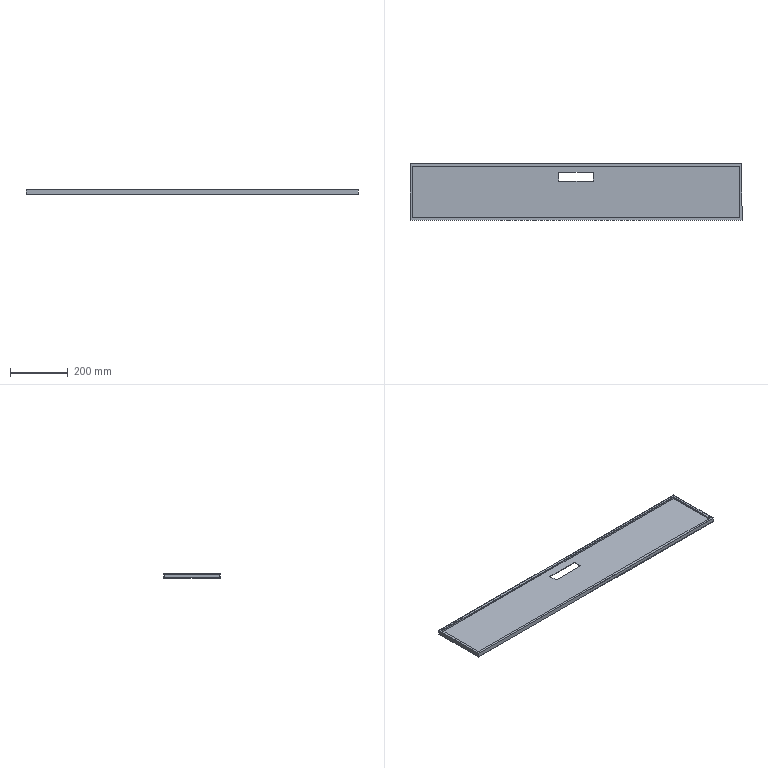Part | SolidWorks | features ICE 2, Extrusion 1, Shell 1 | 1 solid | 20 faces | box 1148 x 195 x 15 mm | volume 541900 mm3 | plane 20
STEP:
#1=CARTESIAN_POINT('',(0.,195.,15.));
#2=VERTEX_POINT('',#1);
#3=CARTESIAN_POINT('',(0.,0.,15.));
#4=VERTEX_POINT('',#3);
#5=CARTESIAN_POINT('',(0.,0.,15.));
#6=DIRECTION('',(0.,-1.,0.));
#7=VECTOR('',#6,1000.);
#8=LINE('',#5,#7);
#9=EDGE_CURVE('',#2,#4,#8,.T.);
#10=ORIENTED_EDGE('',*,*,#9,.T.);
#11=CARTESIAN_POINT('',(1148.,0.,15.));
#12=VERTEX_POINT('',#11);
#13=CARTESIAN_POINT('',(0.,0.,15.));
#14=DIRECTION('',(1.,0.,0.));
#15=VECTOR('',#14,1000.);
#16=LINE('',#13,#15);
#17=EDGE_CURVE('',#4,#12,#16,.T.);
#18=ORIENTED_EDGE('',*,*,#17,.T.);
#19=CARTESIAN_POINT('',(1148.,195.,15.));
#20=VERTEX_POINT('',#19);
#21=CARTESIAN_POINT('',(1148.,0.,15.));
#22=DIRECTION('',(0.,1.,0.));
#23=VECTOR('',#22,1000.);
#24=LINE('',#21,#23);
#25=EDGE_CURVE('',#12,#20,#24,.T.);
#26=ORIENTED_EDGE('',*,*,#25,.T.);
#27=CARTESIAN_POINT('',(0.,195.,15.));
#28=DIRECTION('',(-1.,0.,0.));
#29=VECTOR('',#28,1000.);
#30=LINE('',#27,#29);
#31=EDGE_CURVE('',#20,#2,#30,.T.);
#32=ORIENTED_EDGE('',*,*,#31,.T.);
#33=EDGE_LOOP('',(#10,#18,#26,#32));
#34=FACE_OUTER_BOUND('',#33,.T.);
#35=CARTESIAN_POINT('',(1140.,187.,15.));
#36=VERTEX_POINT('',#35);
#37=CARTESIAN_POINT('',(8.,187.,15.));
#38=VERTEX_POINT('',#37);
#39=CARTESIAN_POINT('',(8.,187.,15.));
#40=DIRECTION('',(-1.,0.,0.));
#41=VECTOR('',#40,1000.);
#42=LINE('',#39,#41);
#43=EDGE_CURVE('',#36,#38,#42,.T.);
#44=ORIENTED_EDGE('',*,*,#43,.F.);
#45=CARTESIAN_POINT('',(1140.,8.,15.));
#46=VERTEX_POINT('',#45);
#47=CARTESIAN_POINT('',(1140.,187.,15.));
#48=DIRECTION('',(0.,1.,0.));
#49=VECTOR('',#48,1000.);
#50=LINE('',#47,#49);
#51=EDGE_CURVE('',#46,#36,#50,.T.);
#52=ORIENTED_EDGE('',*,*,#51,.F.);
#53=CARTESIAN_POINT('',(8.,8.,15.));
#54=VERTEX_POINT('',#53);
#55=CARTESIAN_POINT('',(8.,8.,15.));
#56=DIRECTION('',(1.,0.,0.));
#57=VECTOR('',#56,1000.);
#58=LINE('',#55,#57);
#59=EDGE_CURVE('',#54,#46,#58,.T.);
#60=ORIENTED_EDGE('',*,*,#59,.F.);
#61=CARTESIAN_POINT('',(8.,187.,15.));
#62=DIRECTION('',(0.,-1.,0.));
#63=VECTOR('',#62,1000.);
#64=LINE('',#61,#63);
#65=EDGE_CURVE('',#38,#54,#64,.T.);
#66=ORIENTED_EDGE('',*,*,#65,.F.);
#67=EDGE_LOOP('',(#44,#52,#60,#66));
#68=FACE_BOUND('',#67,.T.);
#69=CARTESIAN_POINT('',(0.,195.,15.));
#70=DIRECTION('',(0.,0.,-1.));
#71=DIRECTION('',(-1.,0.,0.));
#72=AXIS2_PLACEMENT_3D('',#69,#70,#71);
#73=PLANE('',#72);
#74=ADVANCED_FACE('',(#34,#68),#73,.F.);
#75=CARTESIAN_POINT('',(0.,195.,0.));
#76=VERTEX_POINT('',#75);
#77=CARTESIAN_POINT('',(0.,195.,15.));
#78=DIRECTION('',(0.,0.,-1.));
#79=VECTOR('',#78,1000.);
#80=LINE('',#77,#79);
#81=EDGE_CURVE('',#2,#76,#80,.T.);
#82=ORIENTED_EDGE('',*,*,#81,.T.);
#83=CARTESIAN_POINT('',(0.,0.,0.));
#84=VERTEX_POINT('',#83);
#85=CARTESIAN_POINT('',(0.,0.,0.));
#86=DIRECTION('',(0.,-1.,0.));
#87=VECTOR('',#86,1000.);
#88=LINE('',#85,#87);
#89=EDGE_CURVE('',#76,#84,#88,.T.);
#90=ORIENTED_EDGE('',*,*,#89,.T.);
#91=CARTESIAN_POINT('',(0.,0.,15.));
#92=DIRECTION('',(0.,0.,-1.));
#93=VECTOR('',#92,1000.);
#94=LINE('',#91,#93);
#95=EDGE_CURVE('',#4,#84,#94,.T.);
#96=ORIENTED_EDGE('',*,*,#95,.F.);
#97=ORIENTED_EDGE('',*,*,#9,.F.);
#98=EDGE_LOOP('',(#82,#90,#96,#97));
#99=FACE_OUTER_BOUND('',#98,.T.);
#100=CARTESIAN_POINT('',(0.,0.,15.));
#101=DIRECTION('',(1.,0.,0.));
#102=DIRECTION('',(0.,0.,-1.));
#103=AXIS2_PLACEMENT_3D('',#100,#101,#102);
#104=PLANE('',#103);
#105=ADVANCED_FACE('',(#99),#104,.F.);
#106=ORIENTED_EDGE('',*,*,#95,.T.);
#107=CARTESIAN_POINT('',(1148.,0.,0.));
#108=VERTEX_POINT('',#107);
#109=CARTESIAN_POINT('',(0.,0.,0.));
#110=DIRECTION('',(1.,0.,0.));
#111=VECTOR('',#110,1000.);
#112=LINE('',#109,#111);
#113=EDGE_CURVE('',#84,#108,#112,.T.);
#114=ORIENTED_EDGE('',*,*,#113,.T.);
#115=CARTESIAN_POINT('',(1148.,0.,15.));
#116=DIRECTION('',(0.,0.,-1.));
#117=VECTOR('',#116,1000.);
#118=LINE('',#115,#117);
#119=EDGE_CURVE('',#12,#108,#118,.T.);
#120=ORIENTED_EDGE('',*,*,#119,.F.);
#121=ORIENTED_EDGE('',*,*,#17,.F.);
#122=EDGE_LOOP('',(#106,#114,#120,#121));
#123=FACE_OUTER_BOUND('',#122,.T.);
#124=CARTESIAN_POINT('',(0.,0.,15.));
#125=DIRECTION('',(0.,1.,0.));
#126=DIRECTION('',(0.,0.,1.));
#127=AXIS2_PLACEMENT_3D('',#124,#125,#126);
#128=PLANE('',#127);
#129=ADVANCED_FACE('',(#123),#128,.F.);
#130=ORIENTED_EDGE('',*,*,#119,.T.);
#131=CARTESIAN_POINT('',(1148.,195.,0.));
#132=VERTEX_POINT('',#131);
#133=CARTESIAN_POINT('',(1148.,0.,0.));
#134=DIRECTION('',(0.,1.,0.));
#135=VECTOR('',#134,1000.);
#136=LINE('',#133,#135);
#137=EDGE_CURVE('',#108,#132,#136,.T.);
#138=ORIENTED_EDGE('',*,*,#137,.T.);
#139=CARTESIAN_POINT('',(1148.,195.,15.));
#140=DIRECTION('',(0.,0.,-1.));
#141=VECTOR('',#140,1000.);
#142=LINE('',#139,#141);
#143=EDGE_CURVE('',#20,#132,#142,.T.);
#144=ORIENTED_EDGE('',*,*,#143,.F.);
#145=ORIENTED_EDGE('',*,*,#25,.F.);
#146=EDGE_LOOP('',(#130,#138,#144,#145));
#147=FACE_OUTER_BOUND('',#146,.T.);
#148=CARTESIAN_POINT('',(1148.,0.,15.));
#149=DIRECTION('',(-1.,0.,0.));
#150=DIRECTION('',(0.,-1.,0.));
#151=AXIS2_PLACEMENT_3D('',#148,#149,#150);
#152=PLANE('',#151);
#153=ADVANCED_FACE('',(#147),#152,.F.);
#154=ORIENTED_EDGE('',*,*,#143,.T.);
#155=CARTESIAN_POINT('',(0.,195.,0.));
#156=DIRECTION('',(-1.,0.,0.));
#157=VECTOR('',#156,1000.);
#158=LINE('',#155,#157);
#159=EDGE_CURVE('',#132,#76,#158,.T.);
#160=ORIENTED_EDGE('',*,*,#159,.T.);
#161=ORIENTED_EDGE('',*,*,#81,.F.);
#162=ORIENTED_EDGE('',*,*,#31,.F.);
#163=EDGE_LOOP('',(#154,#160,#161,#162));
#164=FACE_OUTER_BOUND('',#163,.T.);
#165=CARTESIAN_POINT('',(0.,195.,15.));
#166=DIRECTION('',(0.,-1.,0.));
#167=DIRECTION('',(0.,0.,-1.));
#168=AXIS2_PLACEMENT_3D('',#165,#166,#167);
#169=PLANE('',#168);
#170=ADVANCED_FACE('',(#164),#169,.F.);
#171=CARTESIAN_POINT('',(634.,165.,0.));
#172=VERTEX_POINT('',#171);
#173=CARTESIAN_POINT('',(634.,135.,0.));
#174=VERTEX_POINT('',#173);
#175=CARTESIAN_POINT('',(634.,165.,0.));
#176=DIRECTION('',(0.,-1.,0.));
#177=VECTOR('',#176,1000.);
#178=LINE('',#175,#177);
#179=EDGE_CURVE('',#172,#174,#178,.T.);
#180=ORIENTED_EDGE('',*,*,#179,.F.);
#181=CARTESIAN_POINT('',(514.,165.,0.));
#182=VERTEX_POINT('',#181);
#183=CARTESIAN_POINT('',(634.,165.,0.));
#184=DIRECTION('',(1.,0.,0.));
#185=VECTOR('',#184,1000.);
#186=LINE('',#183,#185);
#187=EDGE_CURVE('',#182,#172,#186,.T.);
#188=ORIENTED_EDGE('',*,*,#187,.F.);
#189=CARTESIAN_POINT('',(514.,135.,0.));
#190=VERTEX_POINT('',#189);
#191=CARTESIAN_POINT('',(514.,165.,0.));
#192=DIRECTION('',(0.,1.,0.));
#193=VECTOR('',#192,1000.);
#194=LINE('',#191,#193);
#195=EDGE_CURVE('',#190,#182,#194,.T.);
#196=ORIENTED_EDGE('',*,*,#195,.F.);
#197=CARTESIAN_POINT('',(634.,135.,0.));
#198=DIRECTION('',(-1.,0.,0.));
#199=VECTOR('',#198,1000.);
#200=LINE('',#197,#199);
#201=EDGE_CURVE('',#174,#190,#200,.T.);
#202=ORIENTED_EDGE('',*,*,#201,.F.);
#203=EDGE_LOOP('',(#180,#188,#196,#202));
#204=FACE_BOUND('',#203,.T.);
#205=ORIENTED_EDGE('',*,*,#89,.F.);
#206=ORIENTED_EDGE('',*,*,#159,.F.);
#207=ORIENTED_EDGE('',*,*,#137,.F.);
#208=ORIENTED_EDGE('',*,*,#113,.F.);
#209=EDGE_LOOP('',(#205,#206,#207,#208));
#210=FACE_OUTER_BOUND('',#209,.T.);
#211=CARTESIAN_POINT('',(0.,195.,0.));
#212=DIRECTION('',(0.,0.,-1.));
#213=DIRECTION('',(-1.,0.,0.));
#214=AXIS2_PLACEMENT_3D('',#211,#212,#213);
#215=PLANE('',#214);
#216=ADVANCED_FACE('',(#204,#210),#215,.T.);
#217=CARTESIAN_POINT('',(2.,193.,13.));
#218=VERTEX_POINT('',#217);
#219=CARTESIAN_POINT('',(2.,2.,13.));
#220=VERTEX_POINT('',#219);
#221=CARTESIAN_POINT('',(2.,0.,13.));
#222=DIRECTION('',(0.,-1.,0.));
#223=VECTOR('',#222,1000.);
#224=LINE('',#221,#223);
#225=EDGE_CURVE('',#218,#220,#224,.T.);
#226=ORIENTED_EDGE('',*,*,#225,.F.);
#227=CARTESIAN_POINT('',(1146.,193.,13.));
#228=VERTEX_POINT('',#227);
#229=CARTESIAN_POINT('',(0.,193.,13.));
#230=DIRECTION('',(-1.,0.,0.));
#231=VECTOR('',#230,1000.);
#232=LINE('',#229,#231);
#233=EDGE_CURVE('',#228,#218,#232,.T.);
#234=ORIENTED_EDGE('',*,*,#233,.F.);
#235=CARTESIAN_POINT('',(1146.,2.,13.));
#236=VERTEX_POINT('',#235);
#237=CARTESIAN_POINT('',(1146.,0.,13.));
#238=DIRECTION('',(0.,1.,0.));
#239=VECTOR('',#238,1000.);
#240=LINE('',#237,#239);
#241=EDGE_CURVE('',#236,#228,#240,.T.);
#242=ORIENTED_EDGE('',*,*,#241,.F.);
#243=CARTESIAN_POINT('',(0.,2.,13.));
#244=DIRECTION('',(1.,0.,0.));
#245=VECTOR('',#244,1000.);
#246=LINE('',#243,#245);
#247=EDGE_CURVE('',#220,#236,#246,.T.);
#248=ORIENTED_EDGE('',*,*,#247,.F.);
#249=EDGE_LOOP('',(#226,#234,#242,#248));
#250=FACE_OUTER_BOUND('',#249,.T.);
#251=CARTESIAN_POINT('',(1140.,8.,13.));
#252=VERTEX_POINT('',#251);
#253=CARTESIAN_POINT('',(1140.,187.,13.));
#254=VERTEX_POINT('',#253);
#255=CARTESIAN_POINT('',(1140.,187.,13.));
#256=DIRECTION('',(0.,1.,0.));
#257=VECTOR('',#256,1000.);
#258=LINE('',#255,#257);
#259=EDGE_CURVE('',#252,#254,#258,.T.);
#260=ORIENTED_EDGE('',*,*,#259,.T.);
#261=CARTESIAN_POINT('',(8.,187.,13.));
#262=VERTEX_POINT('',#261);
#263=CARTESIAN_POINT('',(8.,187.,13.));
#264=DIRECTION('',(-1.,0.,0.));
#265=VECTOR('',#264,1000.);
#266=LINE('',#263,#265);
#267=EDGE_CURVE('',#254,#262,#266,.T.);
#268=ORIENTED_EDGE('',*,*,#267,.T.);
#269=CARTESIAN_POINT('',(8.,8.,13.));
#270=VERTEX_POINT('',#269);
#271=CARTESIAN_POINT('',(8.,187.,13.));
#272=DIRECTION('',(0.,-1.,0.));
#273=VECTOR('',#272,1000.);
#274=LINE('',#271,#273);
#275=EDGE_CURVE('',#262,#270,#274,.T.);
#276=ORIENTED_EDGE('',*,*,#275,.T.);
#277=CARTESIAN_POINT('',(8.,8.,13.));
#278=DIRECTION('',(1.,0.,0.));
#279=VECTOR('',#278,1000.);
#280=LINE('',#277,#279);
#281=EDGE_CURVE('',#270,#252,#280,.T.);
#282=ORIENTED_EDGE('',*,*,#281,.T.);
#283=EDGE_LOOP('',(#260,#268,#276,#282));
#284=FACE_BOUND('',#283,.T.);
#285=CARTESIAN_POINT('',(0.,0.,13.));
#286=DIRECTION('',(0.,0.,1.));
#287=DIRECTION('',(1.,0.,0.));
#288=AXIS2_PLACEMENT_3D('',#285,#286,#287);
#289=PLANE('',#288);
#290=ADVANCED_FACE('',(#250,#284),#289,.F.);
#291=ORIENTED_EDGE('',*,*,#43,.T.);
#292=CARTESIAN_POINT('',(8.,187.,13.));
#293=DIRECTION('',(0.,0.,1.));
#294=VECTOR('',#293,1000.);
#295=LINE('',#292,#294);
#296=EDGE_CURVE('',#262,#38,#295,.T.);
#297=ORIENTED_EDGE('',*,*,#296,.F.);
#298=ORIENTED_EDGE('',*,*,#267,.F.);
#299=CARTESIAN_POINT('',(1140.,187.,13.));
#300=DIRECTION('',(0.,0.,1.));
#301=VECTOR('',#300,1000.);
#302=LINE('',#299,#301);
#303=EDGE_CURVE('',#254,#36,#302,.T.);
#304=ORIENTED_EDGE('',*,*,#303,.T.);
#305=EDGE_LOOP('',(#291,#297,#298,#304));
#306=FACE_OUTER_BOUND('',#305,.T.);
#307=CARTESIAN_POINT('',(8.,187.,13.));
#308=DIRECTION('',(0.,1.,0.));
#309=DIRECTION('',(0.,0.,1.));
#310=AXIS2_PLACEMENT_3D('',#307,#308,#309);
#311=PLANE('',#310);
#312=ADVANCED_FACE('',(#306),#311,.F.);
#313=ORIENTED_EDGE('',*,*,#51,.T.);
#314=ORIENTED_EDGE('',*,*,#303,.F.);
#315=ORIENTED_EDGE('',*,*,#259,.F.);
#316=CARTESIAN_POINT('',(1140.,8.,13.));
#317=DIRECTION('',(0.,0.,1.));
#318=VECTOR('',#317,1000.);
#319=LINE('',#316,#318);
#320=EDGE_CURVE('',#252,#46,#319,.T.);
#321=ORIENTED_EDGE('',*,*,#320,.T.);
#322=EDGE_LOOP('',(#313,#314,#315,#321));
#323=FACE_OUTER_BOUND('',#322,.T.);
#324=CARTESIAN_POINT('',(1140.,187.,13.));
#325=DIRECTION('',(1.,0.,0.));
#326=DIRECTION('',(0.,0.,-1.));
#327=AXIS2_PLACEMENT_3D('',#324,#325,#326);
#328=PLANE('',#327);
#329=ADVANCED_FACE('',(#323),#328,.F.);
#330=ORIENTED_EDGE('',*,*,#59,.T.);
#331=ORIENTED_EDGE('',*,*,#320,.F.);
#332=ORIENTED_EDGE('',*,*,#281,.F.);
#333=CARTESIAN_POINT('',(8.,8.,13.));
#334=DIRECTION('',(0.,0.,1.));
#335=VECTOR('',#334,1000.);
#336=LINE('',#333,#335);
#337=EDGE_CURVE('',#270,#54,#336,.T.);
#338=ORIENTED_EDGE('',*,*,#337,.T.);
#339=EDGE_LOOP('',(#330,#331,#332,#338));
#340=FACE_OUTER_BOUND('',#339,.T.);
#341=CARTESIAN_POINT('',(8.,8.,13.));
#342=DIRECTION('',(0.,-1.,0.));
#343=DIRECTION('',(1.,0.,0.));
#344=AXIS2_PLACEMENT_3D('',#341,#342,#343);
#345=PLANE('',#344);
#346=ADVANCED_FACE('',(#340),#345,.F.);
#347=ORIENTED_EDGE('',*,*,#65,.T.);
#348=ORIENTED_EDGE('',*,*,#337,.F.);
#349=ORIENTED_EDGE('',*,*,#275,.F.);
#350=ORIENTED_EDGE('',*,*,#296,.T.);
#351=EDGE_LOOP('',(#347,#348,#349,#350));
#352=FACE_OUTER_BOUND('',#351,.T.);
#353=CARTESIAN_POINT('',(8.,187.,13.));
#354=DIRECTION('',(-1.,0.,0.));
#355=DIRECTION('',(0.,-1.,0.));
#356=AXIS2_PLACEMENT_3D('',#353,#354,#355);
#357=PLANE('',#356);
#358=ADVANCED_FACE('',(#352),#357,.F.);
#359=CARTESIAN_POINT('',(514.,165.,2.));
#360=VERTEX_POINT('',#359);
#361=CARTESIAN_POINT('',(634.,165.,2.));
#362=VERTEX_POINT('',#361);
#363=CARTESIAN_POINT('',(0.,165.,2.));
#364=DIRECTION('',(1.,0.,0.));
#365=VECTOR('',#364,1000.);
#366=LINE('',#363,#365);
#367=EDGE_CURVE('',#360,#362,#366,.T.);
#368=ORIENTED_EDGE('',*,*,#367,.T.);
#369=CARTESIAN_POINT('',(634.,135.,2.));
#370=VERTEX_POINT('',#369);
#371=CARTESIAN_POINT('',(634.,195.,2.));
#372=DIRECTION('',(0.,-1.,0.));
#373=VECTOR('',#372,1000.);
#374=LINE('',#371,#373);
#375=EDGE_CURVE('',#362,#370,#374,.T.);
#376=ORIENTED_EDGE('',*,*,#375,.T.);
#377=CARTESIAN_POINT('',(514.,135.,2.));
#378=VERTEX_POINT('',#377);
#379=CARTESIAN_POINT('',(0.,135.,2.));
#380=DIRECTION('',(-1.,0.,0.));
#381=VECTOR('',#380,1000.);
#382=LINE('',#379,#381);
#383=EDGE_CURVE('',#370,#378,#382,.T.);
#384=ORIENTED_EDGE('',*,*,#383,.T.);
#385=CARTESIAN_POINT('',(514.,195.,2.));
#386=DIRECTION('',(0.,1.,0.));
#387=VECTOR('',#386,1000.);
#388=LINE('',#385,#387);
#389=EDGE_CURVE('',#378,#360,#388,.T.);
#390=ORIENTED_EDGE('',*,*,#389,.T.);
#391=EDGE_LOOP('',(#368,#376,#384,#390));
#392=FACE_BOUND('',#391,.T.);
#393=CARTESIAN_POINT('',(2.,193.,2.));
#394=VERTEX_POINT('',#393);
#395=CARTESIAN_POINT('',(2.,2.,2.));
#396=VERTEX_POINT('',#395);
#397=CARTESIAN_POINT('',(2.,195.,2.));
#398=DIRECTION('',(0.,-1.,0.));
#399=VECTOR('',#398,1000.);
#400=LINE('',#397,#399);
#401=EDGE_CURVE('',#394,#396,#400,.T.);
#402=ORIENTED_EDGE('',*,*,#401,.T.);
#403=CARTESIAN_POINT('',(1146.,2.,2.));
#404=VERTEX_POINT('',#403);
#405=CARTESIAN_POINT('',(0.,2.,2.));
#406=DIRECTION('',(1.,0.,0.));
#407=VECTOR('',#406,1000.);
#408=LINE('',#405,#407);
#409=EDGE_CURVE('',#396,#404,#408,.T.);
#410=ORIENTED_EDGE('',*,*,#409,.T.);
#411=CARTESIAN_POINT('',(1146.,193.,2.));
#412=VERTEX_POINT('',#411);
#413=CARTESIAN_POINT('',(1146.,195.,2.));
#414=DIRECTION('',(0.,1.,0.));
#415=VECTOR('',#414,1000.);
#416=LINE('',#413,#415);
#417=EDGE_CURVE('',#404,#412,#416,.T.);
#418=ORIENTED_EDGE('',*,*,#417,.T.);
#419=CARTESIAN_POINT('',(0.,193.,2.));
#420=DIRECTION('',(-1.,0.,0.));
#421=VECTOR('',#420,1000.);
#422=LINE('',#419,#421);
#423=EDGE_CURVE('',#412,#394,#422,.T.);
#424=ORIENTED_EDGE('',*,*,#423,.T.);
#425=EDGE_LOOP('',(#402,#410,#418,#424));
#426=FACE_OUTER_BOUND('',#425,.T.);
#427=CARTESIAN_POINT('',(0.,195.,2.));
#428=DIRECTION('',(0.,0.,-1.));
#429=DIRECTION('',(-1.,0.,0.));
#430=AXIS2_PLACEMENT_3D('',#427,#428,#429);
#431=PLANE('',#430);
#432=ADVANCED_FACE('',(#392,#426),#431,.F.);
#433=CARTESIAN_POINT('',(1146.,193.,15.));
#434=DIRECTION('',(0.,0.,-1.));
#435=VECTOR('',#434,1000.);
#436=LINE('',#433,#435);
#437=EDGE_CURVE('',#228,#412,#436,.T.);
#438=ORIENTED_EDGE('',*,*,#437,.F.);
#439=ORIENTED_EDGE('',*,*,#233,.T.);
#440=CARTESIAN_POINT('',(2.,193.,15.));
#441=DIRECTION('',(0.,0.,-1.));
#442=VECTOR('',#441,1000.);
#443=LINE('',#440,#442);
#444=EDGE_CURVE('',#218,#394,#443,.T.);
#445=ORIENTED_EDGE('',*,*,#444,.T.);
#446=ORIENTED_EDGE('',*,*,#423,.F.);
#447=EDGE_LOOP('',(#438,#439,#445,#446));
#448=FACE_OUTER_BOUND('',#447,.T.);
#449=CARTESIAN_POINT('',(0.,193.,15.));
#450=DIRECTION('',(0.,-1.,0.));
#451=DIRECTION('',(0.,0.,-1.));
#452=AXIS2_PLACEMENT_3D('',#449,#450,#451);
#453=PLANE('',#452);
#454=ADVANCED_FACE('',(#448),#453,.T.);
#455=CARTESIAN_POINT('',(1146.,2.,15.));
#456=DIRECTION('',(0.,0.,-1.));
#457=VECTOR('',#456,1000.);
#458=LINE('',#455,#457);
#459=EDGE_CURVE('',#236,#404,#458,.T.);
#460=ORIENTED_EDGE('',*,*,#459,.F.);
#461=ORIENTED_EDGE('',*,*,#241,.T.);
#462=ORIENTED_EDGE('',*,*,#437,.T.);
#463=ORIENTED_EDGE('',*,*,#417,.F.);
#464=EDGE_LOOP('',(#460,#461,#462,#463));
#465=FACE_OUTER_BOUND('',#464,.T.);
#466=CARTESIAN_POINT('',(1146.,0.,15.));
#467=DIRECTION('',(-1.,0.,0.));
#468=DIRECTION('',(0.,-1.,0.));
#469=AXIS2_PLACEMENT_3D('',#466,#467,#468);
#470=PLANE('',#469);
#471=ADVANCED_FACE('',(#465),#470,.T.);
#472=CARTESIAN_POINT('',(2.,2.,15.));
#473=DIRECTION('',(0.,0.,-1.));
#474=VECTOR('',#473,1000.);
#475=LINE('',#472,#474);
#476=EDGE_CURVE('',#220,#396,#475,.T.);
#477=ORIENTED_EDGE('',*,*,#476,.F.);
#478=ORIENTED_EDGE('',*,*,#247,.T.);
#479=ORIENTED_EDGE('',*,*,#459,.T.);
#480=ORIENTED_EDGE('',*,*,#409,.F.);
#481=EDGE_LOOP('',(#477,#478,#479,#480));
#482=FACE_OUTER_BOUND('',#481,.T.);
#483=CARTESIAN_POINT('',(0.,2.,15.));
#484=DIRECTION('',(0.,1.,0.));
#485=DIRECTION('',(0.,0.,1.));
#486=AXIS2_PLACEMENT_3D('',#483,#484,#485);
#487=PLANE('',#486);
#488=ADVANCED_FACE('',(#482),#487,.T.);
#489=ORIENTED_EDGE('',*,*,#444,.F.);
#490=ORIENTED_EDGE('',*,*,#225,.T.);
#491=ORIENTED_EDGE('',*,*,#476,.T.);
#492=ORIENTED_EDGE('',*,*,#401,.F.);
#493=EDGE_LOOP('',(#489,#490,#491,#492));
#494=FACE_OUTER_BOUND('',#493,.T.);
#495=CARTESIAN_POINT('',(2.,0.,15.));
#496=DIRECTION('',(1.,0.,0.));
#497=DIRECTION('',(0.,0.,-1.));
#498=AXIS2_PLACEMENT_3D('',#495,#496,#497);
#499=PLANE('',#498);
#500=ADVANCED_FACE('',(#494),#499,.T.);
#501=CARTESIAN_POINT('',(634.,165.,10.));
#502=DIRECTION('',(0.,0.,-1.));
#503=VECTOR('',#502,1000.);
#504=LINE('',#501,#503);
#505=EDGE_CURVE('',#362,#172,#504,.T.);
#506=ORIENTED_EDGE('',*,*,#505,.T.);
#507=ORIENTED_EDGE('',*,*,#179,.T.);
#508=CARTESIAN_POINT('',(634.,135.,10.));
#509=DIRECTION('',(0.,0.,-1.));
#510=VECTOR('',#509,1000.);
#511=LINE('',#508,#510);
#512=EDGE_CURVE('',#370,#174,#511,.T.);
#513=ORIENTED_EDGE('',*,*,#512,.F.);
#514=ORIENTED_EDGE('',*,*,#375,.F.);
#515=EDGE_LOOP('',(#506,#507,#513,#514));
#516=FACE_OUTER_BOUND('',#515,.T.);
#517=CARTESIAN_POINT('',(634.,165.,10.));
#518=DIRECTION('',(1.,0.,0.));
#519=DIRECTION('',(0.,0.,-1.));
#520=AXIS2_PLACEMENT_3D('',#517,#518,#519);
#521=PLANE('',#520);
#522=ADVANCED_FACE('',(#516),#521,.F.);
#523=CARTESIAN_POINT('',(514.,165.,10.));
#524=DIRECTION('',(0.,0.,-1.));
#525=VECTOR('',#524,1000.);
#526=LINE('',#523,#525);
#527=EDGE_CURVE('',#360,#182,#526,.T.);
#528=ORIENTED_EDGE('',*,*,#527,.T.);
#529=ORIENTED_EDGE('',*,*,#187,.T.);
#530=ORIENTED_EDGE('',*,*,#505,.F.);
#531=ORIENTED_EDGE('',*,*,#367,.F.);
#532=EDGE_LOOP('',(#528,#529,#530,#531));
#533=FACE_OUTER_BOUND('',#532,.T.);
#534=CARTESIAN_POINT('',(634.,165.,10.));
#535=DIRECTION('',(0.,1.,0.));
#536=DIRECTION('',(-1.,0.,0.));
#537=AXIS2_PLACEMENT_3D('',#534,#535,#536);
#538=PLANE('',#537);
#539=ADVANCED_FACE('',(#533),#538,.F.);
#540=CARTESIAN_POINT('',(514.,135.,10.));
#541=DIRECTION('',(0.,0.,-1.));
#542=VECTOR('',#541,1000.);
#543=LINE('',#540,#542);
#544=EDGE_CURVE('',#378,#190,#543,.T.);
#545=ORIENTED_EDGE('',*,*,#544,.T.);
#546=ORIENTED_EDGE('',*,*,#195,.T.);
#547=ORIENTED_EDGE('',*,*,#527,.F.);
#548=ORIENTED_EDGE('',*,*,#389,.F.);
#549=EDGE_LOOP('',(#545,#546,#547,#548));
#550=FACE_OUTER_BOUND('',#549,.T.);
#551=CARTESIAN_POINT('',(514.,165.,10.));
#552=DIRECTION('',(-1.,0.,0.));
#553=DIRECTION('',(0.,0.,1.));
#554=AXIS2_PLACEMENT_3D('',#551,#552,#553);
#555=PLANE('',#554);
#556=ADVANCED_FACE('',(#550),#555,.F.);
#557=ORIENTED_EDGE('',*,*,#512,.T.);
#558=ORIENTED_EDGE('',*,*,#201,.T.);
#559=ORIENTED_EDGE('',*,*,#544,.F.);
#560=ORIENTED_EDGE('',*,*,#383,.F.);
#561=EDGE_LOOP('',(#557,#558,#559,#560));
#562=FACE_OUTER_BOUND('',#561,.T.);
#563=CARTESIAN_POINT('',(634.,135.,10.));
#564=DIRECTION('',(0.,-1.,0.));
#565=DIRECTION('',(0.,0.,-1.));
#566=AXIS2_PLACEMENT_3D('',#563,#564,#565);
#567=PLANE('',#566);
#568=ADVANCED_FACE('',(#562),#567,.F.);
#569=CLOSED_SHELL('',(#74,#105,#129,#153,#170,#216,#290,#312,#329,#346,#358,#432,#454,#471,#488,#500,#522,#539,#556,#568));
#570=MANIFOLD_SOLID_BREP('',#569);
#571=CARTESIAN_POINT('',(0.,0.,0.));
#572=DIRECTION('',(0.,0.,1.));
#573=DIRECTION('',(1.,0.,0.));
#574=AXIS2_PLACEMENT_3D('',#571,#572,#573);
#575=(LENGTH_UNIT()NAMED_UNIT(*)SI_UNIT(.MILLI.,.METRE.));
#576=UNCERTAINTY_MEASURE_WITH_UNIT(LENGTH_MEASURE(0.00001),#575,'','');
#577=(NAMED_UNIT(*)PLANE_ANGLE_UNIT()SI_UNIT($,.RADIAN.));
#578=(NAMED_UNIT(*)SI_UNIT($,.STERADIAN.)SOLID_ANGLE_UNIT());
#579=(GEOMETRIC_REPRESENTATION_CONTEXT(3)GLOBAL_UNCERTAINTY_ASSIGNED_CONTEXT((#576))GLOBAL_UNIT_ASSIGNED_CONTEXT((#575,#577,#578))REPRESENTATION_CONTEXT('',''));
#580=ADVANCED_BREP_SHAPE_REPRESENTATION('',(#570,#574),#579);